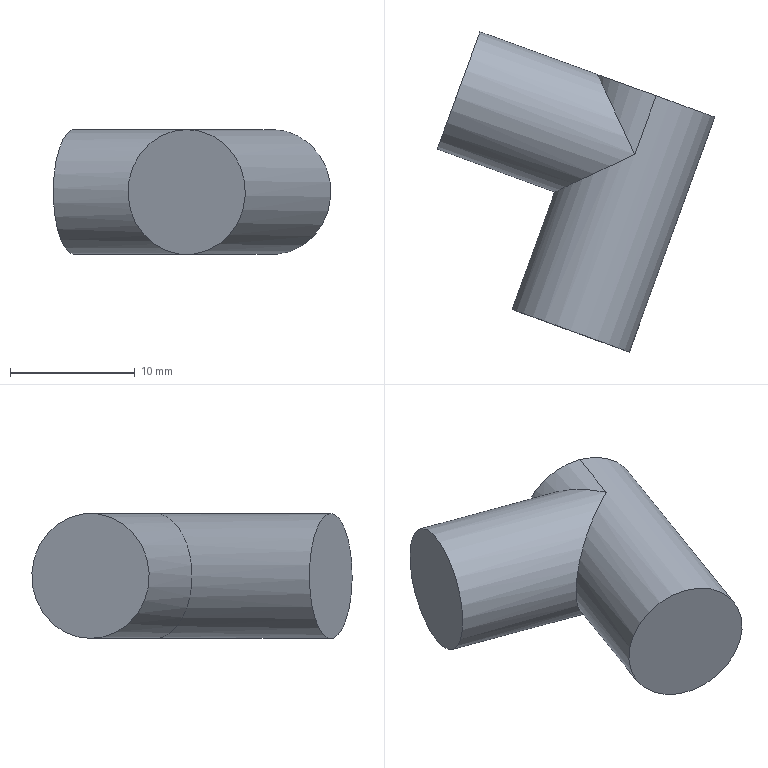Part | NX | features solid 2 | 1 solid | 6 faces | box 22.214 x 25.634 x 10 mm | volume 2416 mm3 | cylinder 3 | plane 3 | commonest cylinder face diameters 10 x3
STEP:
#1=CARTESIAN_POINT('',(1341.985,-267.101,368.5));
#2=VERTEX_POINT('',#1);
#3=CARTESIAN_POINT('',(1341.985,-267.101,378.5));
#4=VERTEX_POINT('',#3);
#5=CARTESIAN_POINT('',(1341.985,-267.101,373.5));
#6=DIRECTION('',(-0.4226,0.9063,0.));
#7=DIRECTION('',(0.9063,0.4226,0.));
#8=AXIS2_PLACEMENT_3D('',#5,#6,#7);
#9=ELLIPSE('',#8,7.071,5.);
#10=EDGE_CURVE('',#2,#4,#9,.T.);
#11=ORIENTED_EDGE('',*,*,#10,.T.);
#12=CARTESIAN_POINT('',(1338.996,-260.692,373.5));
#13=VERTEX_POINT('',#12);
#14=CARTESIAN_POINT('',(1341.985,-267.101,373.5));
#15=DIRECTION('',(-0.9063,-0.4226,0.));
#16=DIRECTION('',(0.4226,-0.9063,0.));
#17=AXIS2_PLACEMENT_3D('',#14,#15,#16);
#18=ELLIPSE('',#17,7.071,5.);
#19=EDGE_CURVE('',#4,#13,#18,.T.);
#20=ORIENTED_EDGE('',*,*,#19,.T.);
#21=CARTESIAN_POINT('',(1341.985,-267.101,373.5));
#22=DIRECTION('',(-0.9063,-0.4226,0.));
#23=DIRECTION('',(0.4226,-0.9063,0.));
#24=AXIS2_PLACEMENT_3D('',#21,#22,#23);
#25=ELLIPSE('',#24,7.071,5.);
#26=EDGE_CURVE('',#13,#2,#25,.T.);
#27=ORIENTED_EDGE('',*,*,#26,.T.);
#28=EDGE_LOOP('',(#11,#20,#27));
#29=FACE_BOUND('',#28,.T.);
#30=CARTESIAN_POINT('',(1327.889,-261.971,368.5));
#31=VERTEX_POINT('',#30);
#32=CARTESIAN_POINT('',(1327.889,-261.971,373.5));
#33=DIRECTION('',(-0.9397,0.342,0.));
#34=DIRECTION('',(0.,0.,-1.));
#35=AXIS2_PLACEMENT_3D('',#32,#33,#34);
#36=CIRCLE('',#35,5.);
#37=EDGE_CURVE('',#31,#31,#36,.T.);
#38=ORIENTED_EDGE('',*,*,#37,.F.);
#39=EDGE_LOOP('',(#38));
#40=FACE_BOUND('',#39,.T.);
#41=CARTESIAN_POINT('',(1323.191,-260.261,373.5));
#42=DIRECTION('',(0.9397,-0.342,0.));
#43=DIRECTION('',(0.,0.,-1.));
#44=AXIS2_PLACEMENT_3D('',#41,#42,#43);
#45=CYLINDRICAL_SURFACE('',#44,5.);
#46=ADVANCED_FACE('',(#29,#40),#45,.T.);
#47=ORIENTED_EDGE('',*,*,#37,.T.);
#48=EDGE_LOOP('',(#47));
#49=FACE_BOUND('',#48,.T.);
#50=CARTESIAN_POINT('',(1327.889,-261.971,373.5));
#51=DIRECTION('',(0.9397,-0.342,0.));
#52=DIRECTION('',(0.,0.,-1.));
#53=AXIS2_PLACEMENT_3D('',#50,#51,#52);
#54=PLANE('',#53);
#55=ADVANCED_FACE('',(#49),#54,.F.);
#56=ORIENTED_EDGE('',*,*,#19,.F.);
#57=ORIENTED_EDGE('',*,*,#10,.F.);
#58=ORIENTED_EDGE('',*,*,#26,.F.);
#59=CARTESIAN_POINT('',(1343.695,-262.403,373.5));
#60=DIRECTION('',(0.342,0.9397,0.));
#61=DIRECTION('',(-0.9397,0.342,0.));
#62=AXIS2_PLACEMENT_3D('',#59,#60,#61);
#63=CIRCLE('',#62,5.);
#64=EDGE_CURVE('',#13,#13,#63,.T.);
#65=ORIENTED_EDGE('',*,*,#64,.F.);
#66=EDGE_LOOP('',(#56,#57,#58,#65));
#67=FACE_BOUND('',#66,.T.);
#68=CARTESIAN_POINT('',(1336.854,-281.196,378.5));
#69=VERTEX_POINT('',#68);
#70=CARTESIAN_POINT('',(1336.854,-281.196,373.5));
#71=DIRECTION('',(0.342,0.9397,0.));
#72=DIRECTION('',(0.,0.,1.));
#73=AXIS2_PLACEMENT_3D('',#70,#71,#72);
#74=CIRCLE('',#73,5.);
#75=EDGE_CURVE('',#69,#69,#74,.T.);
#76=ORIENTED_EDGE('',*,*,#75,.T.);
#77=EDGE_LOOP('',(#76));
#78=FACE_BOUND('',#77,.T.);
#79=CARTESIAN_POINT('',(1348.825,-248.307,373.5));
#80=DIRECTION('',(-0.342,-0.9397,0.));
#81=DIRECTION('',(0.,0.,-1.));
#82=AXIS2_PLACEMENT_3D('',#79,#80,#81);
#83=CYLINDRICAL_SURFACE('',#82,5.);
#84=ADVANCED_FACE('',(#67,#78),#83,.T.);
#85=ORIENTED_EDGE('',*,*,#64,.T.);
#86=EDGE_LOOP('',(#85));
#87=FACE_BOUND('',#86,.T.);
#88=CARTESIAN_POINT('',(1343.695,-262.403,373.5));
#89=DIRECTION('',(-0.342,-0.9397,0.));
#90=DIRECTION('',(0.,0.,-1.));
#91=AXIS2_PLACEMENT_3D('',#88,#89,#90);
#92=PLANE('',#91);
#93=ADVANCED_FACE('',(#87),#92,.F.);
#94=ORIENTED_EDGE('',*,*,#75,.F.);
#95=EDGE_LOOP('',(#94));
#96=FACE_BOUND('',#95,.T.);
#97=CARTESIAN_POINT('',(1336.854,-281.196,373.5));
#98=DIRECTION('',(-0.342,-0.9397,0.));
#99=DIRECTION('',(0.,0.,-1.));
#100=AXIS2_PLACEMENT_3D('',#97,#98,#99);
#101=PLANE('',#100);
#102=ADVANCED_FACE('',(#96),#101,.T.);
#103=CLOSED_SHELL('',(#46,#55,#84,#93,#102));
#104=MANIFOLD_SOLID_BREP('',#103);
#105=(LENGTH_UNIT()NAMED_UNIT(*)SI_UNIT(.MILLI.,.METRE.));
#106=UNCERTAINTY_MEASURE_WITH_UNIT(LENGTH_MEASURE(0.00001),#105,'','');
#107=(NAMED_UNIT(*)PLANE_ANGLE_UNIT()SI_UNIT($,.RADIAN.));
#108=(NAMED_UNIT(*)SI_UNIT($,.STERADIAN.)SOLID_ANGLE_UNIT());
#109=(GEOMETRIC_REPRESENTATION_CONTEXT(3)GLOBAL_UNCERTAINTY_ASSIGNED_CONTEXT((#106))GLOBAL_UNIT_ASSIGNED_CONTEXT((#105,#107,#108))REPRESENTATION_CONTEXT('',''));
#110=ADVANCED_BREP_SHAPE_REPRESENTATION('',(#104),#109);